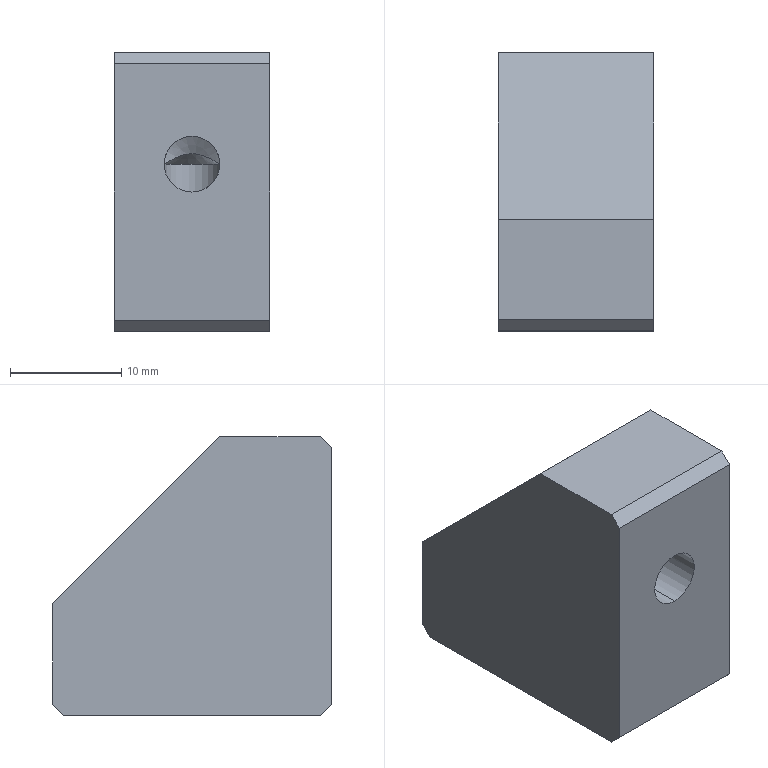Part | SolidWorks | features HoleWzd 2, Chamfer 1, Extrusion 1 | 1 solid | 16 faces | box 14 x 25 x 25 mm | volume 6579 mm3 | plane 10 | cylinder 4 | cone 2 | commonest cylinder face diameters 5 x4
STEP:
#1=CARTESIAN_POINT('',(2.5,15.,15.));
#2=VERTEX_POINT('',#1);
#3=CARTESIAN_POINT('',(0.,12.5,12.5));
#4=VERTEX_POINT('',#3);
#5=CARTESIAN_POINT('',(2.5,15.,15.));
#6=CARTESIAN_POINT('',(2.5,13.536,13.536));
#7=CARTESIAN_POINT('',(1.464,12.5,12.5));
#8=CARTESIAN_POINT('',(0.,12.5,12.5));
#9=(BOUNDED_CURVE()B_SPLINE_CURVE(3,(#5,#6,#7,#8),.UNSPECIFIED.,.F.,.T.)B_SPLINE_CURVE_WITH_KNOTS((4,4),(4.712,6.283),.UNSPECIFIED.)CURVE()GEOMETRIC_REPRESENTATION_ITEM()RATIONAL_B_SPLINE_CURVE((1.,0.8047,0.8047,1.))REPRESENTATION_ITEM(''));
#10=EDGE_CURVE('',#2,#4,#9,.T.);
#11=ORIENTED_EDGE('',*,*,#10,.F.);
#12=CARTESIAN_POINT('',(2.5,15.,0.));
#13=VERTEX_POINT('',#12);
#14=CARTESIAN_POINT('',(2.5,15.,0.));
#15=DIRECTION('',(0.,0.,-1.));
#16=VECTOR('',#15,1000.);
#17=LINE('',#14,#16);
#18=EDGE_CURVE('',#2,#13,#17,.T.);
#19=ORIENTED_EDGE('',*,*,#18,.T.);
#20=CARTESIAN_POINT('',(-2.5,15.,0.));
#21=VERTEX_POINT('',#20);
#22=CARTESIAN_POINT('',(0.,15.,0.));
#23=DIRECTION('',(0.,0.,-1.));
#24=DIRECTION('',(-1.,0.,0.));
#25=AXIS2_PLACEMENT_3D('',#22,#23,#24);
#26=CIRCLE('',#25,2.5);
#27=EDGE_CURVE('',#13,#21,#26,.T.);
#28=ORIENTED_EDGE('',*,*,#27,.T.);
#29=CARTESIAN_POINT('',(-2.5,15.,15.));
#30=VERTEX_POINT('',#29);
#31=CARTESIAN_POINT('',(-2.5,15.,0.));
#32=DIRECTION('',(0.,0.,-1.));
#33=VECTOR('',#32,1000.);
#34=LINE('',#31,#33);
#35=EDGE_CURVE('',#30,#21,#34,.T.);
#36=ORIENTED_EDGE('',*,*,#35,.F.);
#37=CARTESIAN_POINT('',(0.,12.5,12.5));
#38=CARTESIAN_POINT('',(-1.464,12.5,12.5));
#39=CARTESIAN_POINT('',(-2.5,13.536,13.536));
#40=CARTESIAN_POINT('',(-2.5,15.,15.));
#41=(BOUNDED_CURVE()B_SPLINE_CURVE(3,(#37,#38,#39,#40),.UNSPECIFIED.,.F.,.F.)B_SPLINE_CURVE_WITH_KNOTS((4,4),(0.,1.571),.UNSPECIFIED.)CURVE()GEOMETRIC_REPRESENTATION_ITEM()RATIONAL_B_SPLINE_CURVE((1.,0.8047,0.8047,1.))REPRESENTATION_ITEM(''));
#42=EDGE_CURVE('',#4,#30,#41,.T.);
#43=ORIENTED_EDGE('',*,*,#42,.F.);
#44=EDGE_LOOP('',(#11,#19,#28,#36,#43));
#45=FACE_OUTER_BOUND('',#44,.T.);
#46=CARTESIAN_POINT('',(0.,15.,0.));
#47=DIRECTION('',(0.,0.,-1.));
#48=DIRECTION('',(-1.,0.,0.));
#49=AXIS2_PLACEMENT_3D('',#46,#47,#48);
#50=CYLINDRICAL_SURFACE('',#49,2.5);
#51=ADVANCED_FACE('',(#45),#50,.F.);
#52=CARTESIAN_POINT('',(0.,15.,17.5));
#53=VERTEX_POINT('',#52);
#54=CARTESIAN_POINT('',(0.,15.,15.));
#55=DIRECTION('',(0.,-1.,0.));
#56=DIRECTION('',(0.,0.,-1.));
#57=AXIS2_PLACEMENT_3D('',#54,#55,#56);
#58=CIRCLE('',#57,2.5);
#59=EDGE_CURVE('',#53,#30,#58,.T.);
#60=ORIENTED_EDGE('',*,*,#59,.F.);
#61=CARTESIAN_POINT('',(0.,0.,17.5));
#62=VERTEX_POINT('',#61);
#63=CARTESIAN_POINT('',(0.,0.,17.5));
#64=DIRECTION('',(0.,-1.,0.));
#65=VECTOR('',#64,1000.);
#66=LINE('',#63,#65);
#67=EDGE_CURVE('',#53,#62,#66,.T.);
#68=ORIENTED_EDGE('',*,*,#67,.T.);
#69=CARTESIAN_POINT('',(0.,0.,12.5));
#70=VERTEX_POINT('',#69);
#71=CARTESIAN_POINT('',(0.,0.,15.));
#72=DIRECTION('',(0.,-1.,0.));
#73=DIRECTION('',(0.,0.,-1.));
#74=AXIS2_PLACEMENT_3D('',#71,#72,#73);
#75=CIRCLE('',#74,2.5);
#76=EDGE_CURVE('',#62,#70,#75,.T.);
#77=ORIENTED_EDGE('',*,*,#76,.T.);
#78=CARTESIAN_POINT('',(0.,0.,12.5));
#79=DIRECTION('',(0.,-1.,0.));
#80=VECTOR('',#79,1000.);
#81=LINE('',#78,#80);
#82=EDGE_CURVE('',#4,#70,#81,.T.);
#83=ORIENTED_EDGE('',*,*,#82,.F.);
#84=ORIENTED_EDGE('',*,*,#42,.T.);
#85=EDGE_LOOP('',(#60,#68,#77,#83,#84));
#86=FACE_OUTER_BOUND('',#85,.T.);
#87=CARTESIAN_POINT('',(0.,0.,15.));
#88=DIRECTION('',(0.,-1.,0.));
#89=DIRECTION('',(0.,0.,-1.));
#90=AXIS2_PLACEMENT_3D('',#87,#88,#89);
#91=CYLINDRICAL_SURFACE('',#90,2.5);
#92=ADVANCED_FACE('',(#86),#91,.F.);
#93=CARTESIAN_POINT('',(0.,0.,15.));
#94=DIRECTION('',(0.,-1.,0.));
#95=DIRECTION('',(0.,0.,-1.));
#96=AXIS2_PLACEMENT_3D('',#93,#94,#95);
#97=CIRCLE('',#96,2.5);
#98=EDGE_CURVE('',#70,#62,#97,.T.);
#99=ORIENTED_EDGE('',*,*,#98,.F.);
#100=ORIENTED_EDGE('',*,*,#76,.F.);
#101=EDGE_LOOP('',(#99,#100));
#102=FACE_BOUND('',#101,.T.);
#103=CARTESIAN_POINT('',(7.,0.,24.));
#104=VERTEX_POINT('',#103);
#105=CARTESIAN_POINT('',(7.,0.,1.));
#106=VERTEX_POINT('',#105);
#107=CARTESIAN_POINT('',(7.,0.,25.));
#108=DIRECTION('',(0.,0.,-1.));
#109=VECTOR('',#108,1000.);
#110=LINE('',#107,#109);
#111=EDGE_CURVE('',#104,#106,#110,.T.);
#112=ORIENTED_EDGE('',*,*,#111,.F.);
#113=CARTESIAN_POINT('',(-7.,0.,24.));
#114=VERTEX_POINT('',#113);
#115=CARTESIAN_POINT('',(7.,0.,24.));
#116=DIRECTION('',(-1.,0.,0.));
#117=VECTOR('',#116,1000.);
#118=LINE('',#115,#117);
#119=EDGE_CURVE('',#104,#114,#118,.T.);
#120=ORIENTED_EDGE('',*,*,#119,.T.);
#121=CARTESIAN_POINT('',(-7.,0.,1.));
#122=VERTEX_POINT('',#121);
#123=CARTESIAN_POINT('',(-7.,0.,25.));
#124=DIRECTION('',(0.,0.,-1.));
#125=VECTOR('',#124,1000.);
#126=LINE('',#123,#125);
#127=EDGE_CURVE('',#114,#122,#126,.T.);
#128=ORIENTED_EDGE('',*,*,#127,.T.);
#129=CARTESIAN_POINT('',(7.,0.,1.));
#130=DIRECTION('',(1.,0.,0.));
#131=VECTOR('',#130,1000.);
#132=LINE('',#129,#131);
#133=EDGE_CURVE('',#122,#106,#132,.T.);
#134=ORIENTED_EDGE('',*,*,#133,.T.);
#135=EDGE_LOOP('',(#112,#120,#128,#134));
#136=FACE_OUTER_BOUND('',#135,.T.);
#137=CARTESIAN_POINT('',(7.,0.,25.));
#138=DIRECTION('',(0.,1.,0.));
#139=DIRECTION('',(0.,0.,1.));
#140=AXIS2_PLACEMENT_3D('',#137,#138,#139);
#141=PLANE('',#140);
#142=ADVANCED_FACE('',(#102,#136),#141,.F.);
#143=CARTESIAN_POINT('',(0.,15.,0.));
#144=DIRECTION('',(0.,0.,-1.));
#145=DIRECTION('',(-1.,0.,0.));
#146=AXIS2_PLACEMENT_3D('',#143,#144,#145);
#147=CIRCLE('',#146,2.5);
#148=EDGE_CURVE('',#21,#13,#147,.T.);
#149=ORIENTED_EDGE('',*,*,#148,.F.);
#150=ORIENTED_EDGE('',*,*,#27,.F.);
#151=EDGE_LOOP('',(#149,#150));
#152=FACE_BOUND('',#151,.T.);
#153=CARTESIAN_POINT('',(-7.,1.,0.));
#154=VERTEX_POINT('',#153);
#155=CARTESIAN_POINT('',(-7.,24.,0.));
#156=VERTEX_POINT('',#155);
#157=CARTESIAN_POINT('',(-7.,0.,0.));
#158=DIRECTION('',(0.,1.,0.));
#159=VECTOR('',#158,1000.);
#160=LINE('',#157,#159);
#161=EDGE_CURVE('',#154,#156,#160,.T.);
#162=ORIENTED_EDGE('',*,*,#161,.T.);
#163=CARTESIAN_POINT('',(7.,24.,0.));
#164=VERTEX_POINT('',#163);
#165=CARTESIAN_POINT('',(7.,24.,0.));
#166=DIRECTION('',(1.,0.,0.));
#167=VECTOR('',#166,1000.);
#168=LINE('',#165,#167);
#169=EDGE_CURVE('',#156,#164,#168,.T.);
#170=ORIENTED_EDGE('',*,*,#169,.T.);
#171=CARTESIAN_POINT('',(7.,1.,0.));
#172=VERTEX_POINT('',#171);
#173=CARTESIAN_POINT('',(7.,0.,0.));
#174=DIRECTION('',(0.,1.,0.));
#175=VECTOR('',#174,1000.);
#176=LINE('',#173,#175);
#177=EDGE_CURVE('',#172,#164,#176,.T.);
#178=ORIENTED_EDGE('',*,*,#177,.F.);
#179=CARTESIAN_POINT('',(7.,1.,0.));
#180=DIRECTION('',(-1.,0.,0.));
#181=VECTOR('',#180,1000.);
#182=LINE('',#179,#181);
#183=EDGE_CURVE('',#172,#154,#182,.T.);
#184=ORIENTED_EDGE('',*,*,#183,.T.);
#185=EDGE_LOOP('',(#162,#170,#178,#184));
#186=FACE_OUTER_BOUND('',#185,.T.);
#187=CARTESIAN_POINT('',(7.,0.,0.));
#188=DIRECTION('',(0.,0.,1.));
#189=DIRECTION('',(1.,0.,0.));
#190=AXIS2_PLACEMENT_3D('',#187,#188,#189);
#191=PLANE('',#190);
#192=ADVANCED_FACE('',(#152,#186),#191,.F.);
#193=CARTESIAN_POINT('',(7.,25.,1.));
#194=VERTEX_POINT('',#193);
#195=CARTESIAN_POINT('',(7.,25.,10.));
#196=VERTEX_POINT('',#195);
#197=CARTESIAN_POINT('',(7.,25.,0.));
#198=DIRECTION('',(0.,0.,1.));
#199=VECTOR('',#198,1000.);
#200=LINE('',#197,#199);
#201=EDGE_CURVE('',#194,#196,#200,.T.);
#202=ORIENTED_EDGE('',*,*,#201,.F.);
#203=CARTESIAN_POINT('',(-7.,25.,1.));
#204=VERTEX_POINT('',#203);
#205=CARTESIAN_POINT('',(7.,25.,1.));
#206=DIRECTION('',(-1.,0.,0.));
#207=VECTOR('',#206,1000.);
#208=LINE('',#205,#207);
#209=EDGE_CURVE('',#194,#204,#208,.T.);
#210=ORIENTED_EDGE('',*,*,#209,.T.);
#211=CARTESIAN_POINT('',(-7.,25.,10.));
#212=VERTEX_POINT('',#211);
#213=CARTESIAN_POINT('',(-7.,25.,0.));
#214=DIRECTION('',(0.,0.,1.));
#215=VECTOR('',#214,1000.);
#216=LINE('',#213,#215);
#217=EDGE_CURVE('',#204,#212,#216,.T.);
#218=ORIENTED_EDGE('',*,*,#217,.T.);
#219=CARTESIAN_POINT('',(7.,25.,10.));
#220=DIRECTION('',(-1.,0.,0.));
#221=VECTOR('',#220,1000.);
#222=LINE('',#219,#221);
#223=EDGE_CURVE('',#196,#212,#222,.T.);
#224=ORIENTED_EDGE('',*,*,#223,.F.);
#225=EDGE_LOOP('',(#202,#210,#218,#224));
#226=FACE_OUTER_BOUND('',#225,.T.);
#227=CARTESIAN_POINT('',(7.,25.,0.));
#228=DIRECTION('',(0.,-1.,0.));
#229=DIRECTION('',(0.,0.,-1.));
#230=AXIS2_PLACEMENT_3D('',#227,#228,#229);
#231=PLANE('',#230);
#232=ADVANCED_FACE('',(#226),#231,.F.);
#233=CARTESIAN_POINT('',(-7.,10.,25.));
#234=VERTEX_POINT('',#233);
#235=CARTESIAN_POINT('',(-7.,25.,10.));
#236=DIRECTION('',(0.,-0.7071,0.7071));
#237=VECTOR('',#236,1000.);
#238=LINE('',#235,#237);
#239=EDGE_CURVE('',#212,#234,#238,.T.);
#240=ORIENTED_EDGE('',*,*,#239,.T.);
#241=CARTESIAN_POINT('',(7.,10.,25.));
#242=VERTEX_POINT('',#241);
#243=CARTESIAN_POINT('',(7.,10.,25.));
#244=DIRECTION('',(-1.,0.,0.));
#245=VECTOR('',#244,1000.);
#246=LINE('',#243,#245);
#247=EDGE_CURVE('',#242,#234,#246,.T.);
#248=ORIENTED_EDGE('',*,*,#247,.F.);
#249=CARTESIAN_POINT('',(7.,25.,10.));
#250=DIRECTION('',(0.,-0.7071,0.7071));
#251=VECTOR('',#250,1000.);
#252=LINE('',#249,#251);
#253=EDGE_CURVE('',#196,#242,#252,.T.);
#254=ORIENTED_EDGE('',*,*,#253,.F.);
#255=ORIENTED_EDGE('',*,*,#223,.T.);
#256=EDGE_LOOP('',(#240,#248,#254,#255));
#257=FACE_OUTER_BOUND('',#256,.T.);
#258=CARTESIAN_POINT('',(7.,25.,10.));
#259=DIRECTION('',(0.,-0.7071,-0.7071));
#260=DIRECTION('',(0.,0.7071,-0.7071));
#261=AXIS2_PLACEMENT_3D('',#258,#259,#260);
#262=PLANE('',#261);
#263=ADVANCED_FACE('',(#257),#262,.F.);
#264=CARTESIAN_POINT('',(-7.,1.,25.));
#265=VERTEX_POINT('',#264);
#266=CARTESIAN_POINT('',(-7.,10.,25.));
#267=DIRECTION('',(0.,-1.,0.));
#268=VECTOR('',#267,1000.);
#269=LINE('',#266,#268);
#270=EDGE_CURVE('',#234,#265,#269,.T.);
#271=ORIENTED_EDGE('',*,*,#270,.T.);
#272=CARTESIAN_POINT('',(7.,1.,25.));
#273=VERTEX_POINT('',#272);
#274=CARTESIAN_POINT('',(7.,1.,25.));
#275=DIRECTION('',(1.,0.,0.));
#276=VECTOR('',#275,1000.);
#277=LINE('',#274,#276);
#278=EDGE_CURVE('',#265,#273,#277,.T.);
#279=ORIENTED_EDGE('',*,*,#278,.T.);
#280=CARTESIAN_POINT('',(7.,10.,25.));
#281=DIRECTION('',(0.,-1.,0.));
#282=VECTOR('',#281,1000.);
#283=LINE('',#280,#282);
#284=EDGE_CURVE('',#242,#273,#283,.T.);
#285=ORIENTED_EDGE('',*,*,#284,.F.);
#286=ORIENTED_EDGE('',*,*,#247,.T.);
#287=EDGE_LOOP('',(#271,#279,#285,#286));
#288=FACE_OUTER_BOUND('',#287,.T.);
#289=CARTESIAN_POINT('',(7.,10.,25.));
#290=DIRECTION('',(0.,0.,-1.));
#291=DIRECTION('',(-1.,0.,0.));
#292=AXIS2_PLACEMENT_3D('',#289,#290,#291);
#293=PLANE('',#292);
#294=ADVANCED_FACE('',(#288),#293,.F.);
#295=ORIENTED_EDGE('',*,*,#284,.T.);
#296=CARTESIAN_POINT('',(7.,-12.,12.));
#297=DIRECTION('',(0.,-0.7071,-0.7071));
#298=VECTOR('',#297,1000.);
#299=LINE('',#296,#298);
#300=EDGE_CURVE('',#273,#104,#299,.T.);
#301=ORIENTED_EDGE('',*,*,#300,.T.);
#302=ORIENTED_EDGE('',*,*,#111,.T.);
#303=CARTESIAN_POINT('',(7.,0.5,0.5));
#304=DIRECTION('',(0.,0.7071,-0.7071));
#305=VECTOR('',#304,1000.);
#306=LINE('',#303,#305);
#307=EDGE_CURVE('',#106,#172,#306,.T.);
#308=ORIENTED_EDGE('',*,*,#307,.T.);
#309=ORIENTED_EDGE('',*,*,#177,.T.);
#310=CARTESIAN_POINT('',(7.,12.,-12.));
#311=DIRECTION('',(0.,0.7071,0.7071));
#312=VECTOR('',#311,1000.);
#313=LINE('',#310,#312);
#314=EDGE_CURVE('',#164,#194,#313,.T.);
#315=ORIENTED_EDGE('',*,*,#314,.T.);
#316=ORIENTED_EDGE('',*,*,#201,.T.);
#317=ORIENTED_EDGE('',*,*,#253,.T.);
#318=EDGE_LOOP('',(#295,#301,#302,#308,#309,#315,#316,#317));
#319=FACE_OUTER_BOUND('',#318,.T.);
#320=CARTESIAN_POINT('',(7.,0.,0.));
#321=DIRECTION('',(1.,0.,0.));
#322=DIRECTION('',(0.,0.,-1.));
#323=AXIS2_PLACEMENT_3D('',#320,#321,#322);
#324=PLANE('',#323);
#325=ADVANCED_FACE('',(#319),#324,.T.);
#326=ORIENTED_EDGE('',*,*,#127,.F.);
#327=CARTESIAN_POINT('',(-7.,0.,24.));
#328=DIRECTION('',(0.,0.7071,0.7071));
#329=VECTOR('',#328,1000.);
#330=LINE('',#327,#329);
#331=EDGE_CURVE('',#114,#265,#330,.T.);
#332=ORIENTED_EDGE('',*,*,#331,.T.);
#333=ORIENTED_EDGE('',*,*,#270,.F.);
#334=ORIENTED_EDGE('',*,*,#239,.F.);
#335=ORIENTED_EDGE('',*,*,#217,.F.);
#336=CARTESIAN_POINT('',(-7.,25.,1.));
#337=DIRECTION('',(0.,-0.7071,-0.7071));
#338=VECTOR('',#337,1000.);
#339=LINE('',#336,#338);
#340=EDGE_CURVE('',#204,#156,#339,.T.);
#341=ORIENTED_EDGE('',*,*,#340,.T.);
#342=ORIENTED_EDGE('',*,*,#161,.F.);
#343=CARTESIAN_POINT('',(-7.,1.,0.));
#344=DIRECTION('',(0.,-0.7071,0.7071));
#345=VECTOR('',#344,1000.);
#346=LINE('',#343,#345);
#347=EDGE_CURVE('',#154,#122,#346,.T.);
#348=ORIENTED_EDGE('',*,*,#347,.T.);
#349=EDGE_LOOP('',(#326,#332,#333,#334,#335,#341,#342,#348));
#350=FACE_OUTER_BOUND('',#349,.T.);
#351=CARTESIAN_POINT('',(-7.,0.,0.));
#352=DIRECTION('',(1.,0.,0.));
#353=DIRECTION('',(0.,0.,-1.));
#354=AXIS2_PLACEMENT_3D('',#351,#352,#353);
#355=PLANE('',#354);
#356=ADVANCED_FACE('',(#350),#355,.F.);
#357=CARTESIAN_POINT('',(0.,15.,15.));
#358=DIRECTION('',(0.,-1.,0.));
#359=DIRECTION('',(0.,0.,-1.));
#360=AXIS2_PLACEMENT_3D('',#357,#358,#359);
#361=CIRCLE('',#360,2.5);
#362=EDGE_CURVE('',#2,#53,#361,.T.);
#363=ORIENTED_EDGE('',*,*,#362,.T.);
#364=ORIENTED_EDGE('',*,*,#59,.T.);
#365=CARTESIAN_POINT('',(-2.5,15.,15.));
#366=CARTESIAN_POINT('',(-2.316,15.11,15.11));
#367=CARTESIAN_POINT('',(-2.13,15.218,15.218));
#368=CARTESIAN_POINT('',(-1.747,15.425,15.425));
#369=CARTESIAN_POINT('',(-1.551,15.524,15.524));
#370=CARTESIAN_POINT('',(-1.14,15.704,15.704));
#371=CARTESIAN_POINT('',(-0.927,15.784,15.784));
#372=CARTESIAN_POINT('',(-0.5878,15.873,15.873));
#373=CARTESIAN_POINT('',(-0.4706,15.897,15.897));
#374=CARTESIAN_POINT('',(-0.2349,15.93,15.93));
#375=CARTESIAN_POINT('',(-0.1155,15.939,15.939));
#376=CARTESIAN_POINT('',(0.2478,15.938,15.938));
#377=CARTESIAN_POINT('',(0.4854,15.901,15.901));
#378=CARTESIAN_POINT('',(0.9389,15.78,15.78));
#379=CARTESIAN_POINT('',(1.149,15.7,15.7));
#380=CARTESIAN_POINT('',(1.757,15.433,15.433));
#381=CARTESIAN_POINT('',(2.134,15.22,15.22));
#382=CARTESIAN_POINT('',(2.5,15.,15.));
#383=B_SPLINE_CURVE_WITH_KNOTS('',3,(#365,#366,#367,#368,#369,#370,#371,#372,#373,#374,#375,#376,#377,#378,#379,#380,#381,#382),.UNSPECIFIED.,.F.,.F.,(4,2,2,2,2,2,2,2,4),(0.000000262,0.0007226,0.001445,0.002167,0.002528,0.00289,0.003612,0.004334,0.005779),.UNSPECIFIED.);
#384=EDGE_CURVE('',#30,#2,#383,.T.);
#385=ORIENTED_EDGE('',*,*,#384,.T.);
#386=EDGE_LOOP('',(#363,#364,#385));
#387=FACE_OUTER_BOUND('',#386,.T.);
#388=CARTESIAN_POINT('',(0.,15.,15.));
#389=DIRECTION('',(0.,-1.,0.));
#390=DIRECTION('',(0.,0.,-1.));
#391=AXIS2_PLACEMENT_3D('',#388,#389,#390);
#392=CONICAL_SURFACE('',#391,2.5,1.03);
#393=ADVANCED_FACE('',(#387),#392,.F.);
#394=ORIENTED_EDGE('',*,*,#67,.F.);
#395=ORIENTED_EDGE('',*,*,#362,.F.);
#396=ORIENTED_EDGE('',*,*,#10,.T.);
#397=ORIENTED_EDGE('',*,*,#82,.T.);
#398=ORIENTED_EDGE('',*,*,#98,.T.);
#399=EDGE_LOOP('',(#394,#395,#396,#397,#398));
#400=FACE_OUTER_BOUND('',#399,.T.);
#401=CARTESIAN_POINT('',(0.,0.,15.));
#402=DIRECTION('',(0.,-1.,0.));
#403=DIRECTION('',(0.,0.,-1.));
#404=AXIS2_PLACEMENT_3D('',#401,#402,#403);
#405=CYLINDRICAL_SURFACE('',#404,2.5);
#406=ADVANCED_FACE('',(#400),#405,.F.);
#407=ORIENTED_EDGE('',*,*,#18,.F.);
#408=CARTESIAN_POINT('',(0.,15.,15.));
#409=DIRECTION('',(0.,0.,-1.));
#410=DIRECTION('',(-1.,0.,0.));
#411=AXIS2_PLACEMENT_3D('',#408,#409,#410);
#412=CIRCLE('',#411,2.5);
#413=EDGE_CURVE('',#30,#2,#412,.T.);
#414=ORIENTED_EDGE('',*,*,#413,.F.);
#415=ORIENTED_EDGE('',*,*,#35,.T.);
#416=ORIENTED_EDGE('',*,*,#148,.T.);
#417=EDGE_LOOP('',(#407,#414,#415,#416));
#418=FACE_OUTER_BOUND('',#417,.T.);
#419=CARTESIAN_POINT('',(0.,15.,0.));
#420=DIRECTION('',(0.,0.,-1.));
#421=DIRECTION('',(-1.,0.,0.));
#422=AXIS2_PLACEMENT_3D('',#419,#420,#421);
#423=CYLINDRICAL_SURFACE('',#422,2.5);
#424=ADVANCED_FACE('',(#418),#423,.F.);
#425=ORIENTED_EDGE('',*,*,#413,.T.);
#426=ORIENTED_EDGE('',*,*,#384,.F.);
#427=EDGE_LOOP('',(#425,#426));
#428=FACE_OUTER_BOUND('',#427,.T.);
#429=CARTESIAN_POINT('',(0.,15.,15.));
#430=DIRECTION('',(0.,0.,-1.));
#431=DIRECTION('',(-1.,0.,0.));
#432=AXIS2_PLACEMENT_3D('',#429,#430,#431);
#433=CONICAL_SURFACE('',#432,2.5,1.03);
#434=ADVANCED_FACE('',(#428),#433,.F.);
#435=ORIENTED_EDGE('',*,*,#300,.F.);
#436=ORIENTED_EDGE('',*,*,#278,.F.);
#437=ORIENTED_EDGE('',*,*,#331,.F.);
#438=ORIENTED_EDGE('',*,*,#119,.F.);
#439=EDGE_LOOP('',(#435,#436,#437,#438));
#440=FACE_OUTER_BOUND('',#439,.T.);
#441=CARTESIAN_POINT('',(7.,0.,24.));
#442=DIRECTION('',(0.,0.7071,-0.7071));
#443=DIRECTION('',(-1.,0.,0.));
#444=AXIS2_PLACEMENT_3D('',#441,#442,#443);
#445=PLANE('',#444);
#446=ADVANCED_FACE('',(#440),#445,.F.);
#447=ORIENTED_EDGE('',*,*,#314,.F.);
#448=ORIENTED_EDGE('',*,*,#169,.F.);
#449=ORIENTED_EDGE('',*,*,#340,.F.);
#450=ORIENTED_EDGE('',*,*,#209,.F.);
#451=EDGE_LOOP('',(#447,#448,#449,#450));
#452=FACE_OUTER_BOUND('',#451,.T.);
#453=CARTESIAN_POINT('',(7.,25.,1.));
#454=DIRECTION('',(0.,-0.7071,0.7071));
#455=DIRECTION('',(-1.,0.,0.));
#456=AXIS2_PLACEMENT_3D('',#453,#454,#455);
#457=PLANE('',#456);
#458=ADVANCED_FACE('',(#452),#457,.F.);
#459=ORIENTED_EDGE('',*,*,#307,.F.);
#460=ORIENTED_EDGE('',*,*,#133,.F.);
#461=ORIENTED_EDGE('',*,*,#347,.F.);
#462=ORIENTED_EDGE('',*,*,#183,.F.);
#463=EDGE_LOOP('',(#459,#460,#461,#462));
#464=FACE_OUTER_BOUND('',#463,.T.);
#465=CARTESIAN_POINT('',(7.,1.,0.));
#466=DIRECTION('',(0.,0.7071,0.7071));
#467=DIRECTION('',(-1.,0.,0.));
#468=AXIS2_PLACEMENT_3D('',#465,#466,#467);
#469=PLANE('',#468);
#470=ADVANCED_FACE('',(#464),#469,.F.);
#471=CLOSED_SHELL('',(#51,#92,#142,#192,#232,#263,#294,#325,#356,#393,#406,#424,#434,#446,#458,#470));
#472=MANIFOLD_SOLID_BREP('',#471);
#473=CARTESIAN_POINT('',(0.,0.,0.));
#474=DIRECTION('',(0.,0.,1.));
#475=DIRECTION('',(1.,0.,0.));
#476=AXIS2_PLACEMENT_3D('',#473,#474,#475);
#477=(LENGTH_UNIT()NAMED_UNIT(*)SI_UNIT(.MILLI.,.METRE.));
#478=UNCERTAINTY_MEASURE_WITH_UNIT(LENGTH_MEASURE(0.00001),#477,'','');
#479=(NAMED_UNIT(*)PLANE_ANGLE_UNIT()SI_UNIT($,.RADIAN.));
#480=(NAMED_UNIT(*)SI_UNIT($,.STERADIAN.)SOLID_ANGLE_UNIT());
#481=(GEOMETRIC_REPRESENTATION_CONTEXT(3)GLOBAL_UNCERTAINTY_ASSIGNED_CONTEXT((#478))GLOBAL_UNIT_ASSIGNED_CONTEXT((#477,#479,#480))REPRESENTATION_CONTEXT('',''));
#482=ADVANCED_BREP_SHAPE_REPRESENTATION('',(#472,#476),#481);